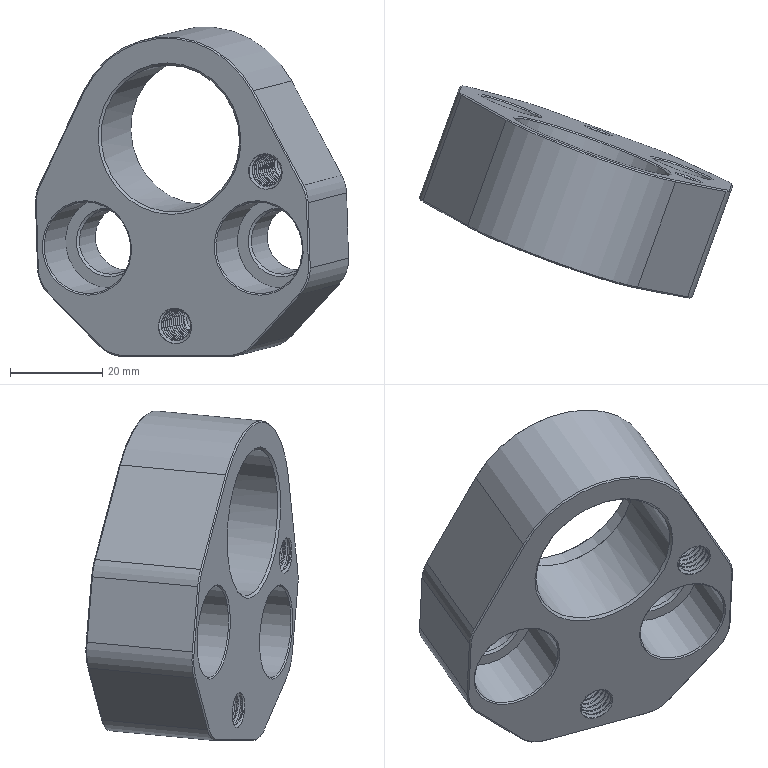Part | NX | features solid 2 | 1 solid | 82 faces | box 67.946 x 46.06 x 71.561 mm | volume 51236 mm3 | plane 30 | cone 29 | cylinder 19 | spline 4 | commonest cylinder face diameters 16 x6 5.8 x2 6.918 x2 8 x2 14 x2 20 x2